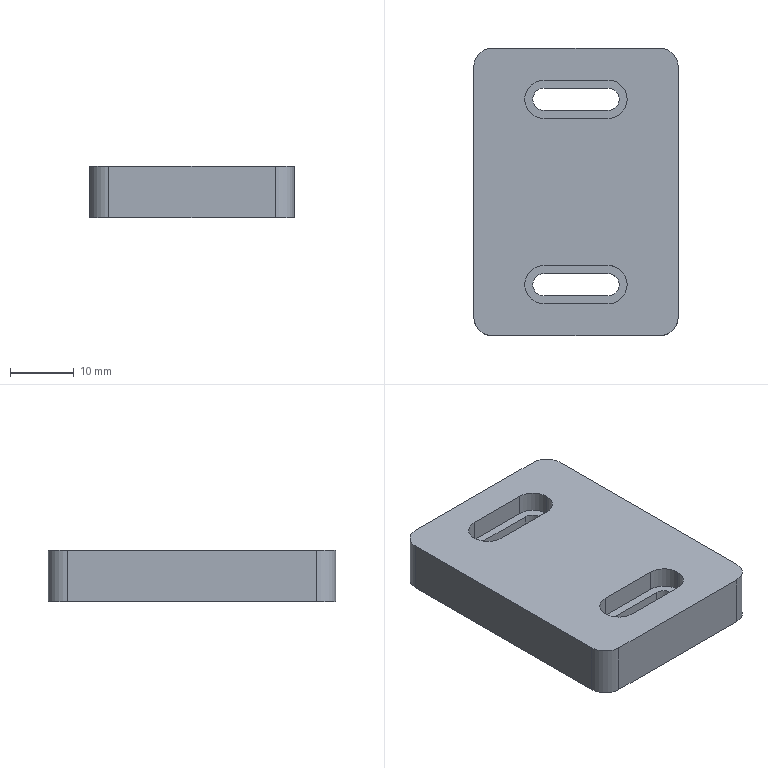Part | SolidWorks | features ICE 2, Extrusion 1, Fillet 1 | 1 solid | 32 faces | box 32 x 45 x 8 mm | volume 10456 mm3 | cylinder 16 | plane 16 | commonest cylinder face diameters 6 x10 3.5 x6
STEP:
#1=CARTESIAN_POINT('',(8.,-14.5,4.7));
#2=VERTEX_POINT('',#1);
#3=CARTESIAN_POINT('',(5.,-11.5,4.7));
#4=VERTEX_POINT('',#3);
#5=CARTESIAN_POINT('',(5.,-14.5,4.7));
#6=DIRECTION('',(0.,0.,1.));
#7=DIRECTION('',(1.,0.,0.));
#8=AXIS2_PLACEMENT_3D('',#5,#6,#7);
#9=CIRCLE('',#8,3.);
#10=EDGE_CURVE('',#2,#4,#9,.T.);
#11=ORIENTED_EDGE('',*,*,#10,.F.);
#12=CARTESIAN_POINT('',(8.,-14.5,8.));
#13=VERTEX_POINT('',#12);
#14=CARTESIAN_POINT('',(8.,-14.5,4.7));
#15=DIRECTION('',(0.,0.,1.));
#16=VECTOR('',#15,1000.);
#17=LINE('',#14,#16);
#18=EDGE_CURVE('',#2,#13,#17,.T.);
#19=ORIENTED_EDGE('',*,*,#18,.T.);
#20=CARTESIAN_POINT('',(5.,-11.5,8.));
#21=VERTEX_POINT('',#20);
#22=CARTESIAN_POINT('',(5.,-14.5,8.));
#23=DIRECTION('',(0.,0.,1.));
#24=DIRECTION('',(1.,0.,0.));
#25=AXIS2_PLACEMENT_3D('',#22,#23,#24);
#26=CIRCLE('',#25,3.);
#27=EDGE_CURVE('',#13,#21,#26,.T.);
#28=ORIENTED_EDGE('',*,*,#27,.T.);
#29=CARTESIAN_POINT('',(5.,-11.5,4.7));
#30=DIRECTION('',(0.,0.,1.));
#31=VECTOR('',#30,1000.);
#32=LINE('',#29,#31);
#33=EDGE_CURVE('',#4,#21,#32,.T.);
#34=ORIENTED_EDGE('',*,*,#33,.F.);
#35=EDGE_LOOP('',(#11,#19,#28,#34));
#36=FACE_OUTER_BOUND('',#35,.T.);
#37=CARTESIAN_POINT('',(5.,-14.5,4.7));
#38=DIRECTION('',(0.,0.,1.));
#39=DIRECTION('',(1.,0.,0.));
#40=AXIS2_PLACEMENT_3D('',#37,#38,#39);
#41=CYLINDRICAL_SURFACE('',#40,3.);
#42=ADVANCED_FACE('',(#36),#41,.F.);
#43=CARTESIAN_POINT('',(8.,14.5,4.7));
#44=VERTEX_POINT('',#43);
#45=CARTESIAN_POINT('',(5.,17.5,4.7));
#46=VERTEX_POINT('',#45);
#47=CARTESIAN_POINT('',(5.,14.5,4.7));
#48=DIRECTION('',(0.,0.,1.));
#49=DIRECTION('',(1.,0.,0.));
#50=AXIS2_PLACEMENT_3D('',#47,#48,#49);
#51=CIRCLE('',#50,3.);
#52=EDGE_CURVE('',#44,#46,#51,.T.);
#53=ORIENTED_EDGE('',*,*,#52,.F.);
#54=CARTESIAN_POINT('',(8.,14.5,8.));
#55=VERTEX_POINT('',#54);
#56=CARTESIAN_POINT('',(8.,14.5,4.7));
#57=DIRECTION('',(0.,0.,1.));
#58=VECTOR('',#57,1000.);
#59=LINE('',#56,#58);
#60=EDGE_CURVE('',#44,#55,#59,.T.);
#61=ORIENTED_EDGE('',*,*,#60,.T.);
#62=CARTESIAN_POINT('',(5.,17.5,8.));
#63=VERTEX_POINT('',#62);
#64=CARTESIAN_POINT('',(5.,14.5,8.));
#65=DIRECTION('',(0.,0.,1.));
#66=DIRECTION('',(1.,0.,0.));
#67=AXIS2_PLACEMENT_3D('',#64,#65,#66);
#68=CIRCLE('',#67,3.);
#69=EDGE_CURVE('',#55,#63,#68,.T.);
#70=ORIENTED_EDGE('',*,*,#69,.T.);
#71=CARTESIAN_POINT('',(5.,17.5,4.7));
#72=DIRECTION('',(0.,0.,1.));
#73=VECTOR('',#72,1000.);
#74=LINE('',#71,#73);
#75=EDGE_CURVE('',#46,#63,#74,.T.);
#76=ORIENTED_EDGE('',*,*,#75,.F.);
#77=EDGE_LOOP('',(#53,#61,#70,#76));
#78=FACE_OUTER_BOUND('',#77,.T.);
#79=CARTESIAN_POINT('',(5.,14.5,4.7));
#80=DIRECTION('',(0.,0.,1.));
#81=DIRECTION('',(1.,0.,0.));
#82=AXIS2_PLACEMENT_3D('',#79,#80,#81);
#83=CYLINDRICAL_SURFACE('',#82,3.);
#84=ADVANCED_FACE('',(#78),#83,.F.);
#85=CARTESIAN_POINT('',(6.75,14.5,0.));
#86=VERTEX_POINT('',#85);
#87=CARTESIAN_POINT('',(5.,16.25,0.));
#88=VERTEX_POINT('',#87);
#89=CARTESIAN_POINT('',(5.,14.5,0.));
#90=DIRECTION('',(0.,0.,1.));
#91=DIRECTION('',(1.,0.,0.));
#92=AXIS2_PLACEMENT_3D('',#89,#90,#91);
#93=CIRCLE('',#92,1.75);
#94=EDGE_CURVE('',#86,#88,#93,.T.);
#95=ORIENTED_EDGE('',*,*,#94,.F.);
#96=CARTESIAN_POINT('',(6.75,14.5,4.7));
#97=VERTEX_POINT('',#96);
#98=CARTESIAN_POINT('',(6.75,14.5,0.));
#99=DIRECTION('',(0.,0.,1.));
#100=VECTOR('',#99,1000.);
#101=LINE('',#98,#100);
#102=EDGE_CURVE('',#86,#97,#101,.T.);
#103=ORIENTED_EDGE('',*,*,#102,.T.);
#104=CARTESIAN_POINT('',(5.,16.25,4.7));
#105=VERTEX_POINT('',#104);
#106=CARTESIAN_POINT('',(5.,14.5,4.7));
#107=DIRECTION('',(0.,0.,-1.));
#108=DIRECTION('',(1.,0.,0.));
#109=AXIS2_PLACEMENT_3D('',#106,#107,#108);
#110=CIRCLE('',#109,1.75);
#111=EDGE_CURVE('',#105,#97,#110,.T.);
#112=ORIENTED_EDGE('',*,*,#111,.F.);
#113=CARTESIAN_POINT('',(5.,16.25,0.));
#114=DIRECTION('',(0.,0.,1.));
#115=VECTOR('',#114,1000.);
#116=LINE('',#113,#115);
#117=EDGE_CURVE('',#88,#105,#116,.T.);
#118=ORIENTED_EDGE('',*,*,#117,.F.);
#119=EDGE_LOOP('',(#95,#103,#112,#118));
#120=FACE_OUTER_BOUND('',#119,.T.);
#121=CARTESIAN_POINT('',(5.,14.5,0.));
#122=DIRECTION('',(0.,0.,1.));
#123=DIRECTION('',(1.,0.,0.));
#124=AXIS2_PLACEMENT_3D('',#121,#122,#123);
#125=CYLINDRICAL_SURFACE('',#124,1.75);
#126=ADVANCED_FACE('',(#120),#125,.F.);
#127=CARTESIAN_POINT('',(6.75,-14.5,0.));
#128=VERTEX_POINT('',#127);
#129=CARTESIAN_POINT('',(5.,-12.75,0.));
#130=VERTEX_POINT('',#129);
#131=CARTESIAN_POINT('',(5.,-14.5,0.));
#132=DIRECTION('',(0.,0.,1.));
#133=DIRECTION('',(1.,0.,0.));
#134=AXIS2_PLACEMENT_3D('',#131,#132,#133);
#135=CIRCLE('',#134,1.75);
#136=EDGE_CURVE('',#128,#130,#135,.T.);
#137=ORIENTED_EDGE('',*,*,#136,.F.);
#138=CARTESIAN_POINT('',(6.75,-14.5,4.7));
#139=VERTEX_POINT('',#138);
#140=CARTESIAN_POINT('',(6.75,-14.5,0.));
#141=DIRECTION('',(0.,0.,1.));
#142=VECTOR('',#141,1000.);
#143=LINE('',#140,#142);
#144=EDGE_CURVE('',#128,#139,#143,.T.);
#145=ORIENTED_EDGE('',*,*,#144,.T.);
#146=CARTESIAN_POINT('',(5.,-12.75,4.7));
#147=VERTEX_POINT('',#146);
#148=CARTESIAN_POINT('',(5.,-14.5,4.7));
#149=DIRECTION('',(0.,0.,-1.));
#150=DIRECTION('',(1.,0.,0.));
#151=AXIS2_PLACEMENT_3D('',#148,#149,#150);
#152=CIRCLE('',#151,1.75);
#153=EDGE_CURVE('',#147,#139,#152,.T.);
#154=ORIENTED_EDGE('',*,*,#153,.F.);
#155=CARTESIAN_POINT('',(5.,-12.75,0.));
#156=DIRECTION('',(0.,0.,1.));
#157=VECTOR('',#156,1000.);
#158=LINE('',#155,#157);
#159=EDGE_CURVE('',#130,#147,#158,.T.);
#160=ORIENTED_EDGE('',*,*,#159,.F.);
#161=EDGE_LOOP('',(#137,#145,#154,#160));
#162=FACE_OUTER_BOUND('',#161,.T.);
#163=CARTESIAN_POINT('',(5.,-14.5,0.));
#164=DIRECTION('',(0.,0.,1.));
#165=DIRECTION('',(1.,0.,0.));
#166=AXIS2_PLACEMENT_3D('',#163,#164,#165);
#167=CYLINDRICAL_SURFACE('',#166,1.75);
#168=ADVANCED_FACE('',(#162),#167,.F.);
#169=CARTESIAN_POINT('',(-5.,-16.25,4.7));
#170=VERTEX_POINT('',#169);
#171=CARTESIAN_POINT('',(-5.,-12.75,4.7));
#172=VERTEX_POINT('',#171);
#173=CARTESIAN_POINT('',(-5.,-14.5,4.7));
#174=DIRECTION('',(0.,0.,-1.));
#175=DIRECTION('',(1.,0.,0.));
#176=AXIS2_PLACEMENT_3D('',#173,#174,#175);
#177=CIRCLE('',#176,1.75);
#178=EDGE_CURVE('',#170,#172,#177,.T.);
#179=ORIENTED_EDGE('',*,*,#178,.F.);
#180=CARTESIAN_POINT('',(-5.,-16.25,0.));
#181=VERTEX_POINT('',#180);
#182=CARTESIAN_POINT('',(-5.,-16.25,0.));
#183=DIRECTION('',(0.,0.,1.));
#184=VECTOR('',#183,1000.);
#185=LINE('',#182,#184);
#186=EDGE_CURVE('',#181,#170,#185,.T.);
#187=ORIENTED_EDGE('',*,*,#186,.F.);
#188=CARTESIAN_POINT('',(-5.,-12.75,0.));
#189=VERTEX_POINT('',#188);
#190=CARTESIAN_POINT('',(-5.,-14.5,0.));
#191=DIRECTION('',(0.,0.,1.));
#192=DIRECTION('',(1.,0.,0.));
#193=AXIS2_PLACEMENT_3D('',#190,#191,#192);
#194=CIRCLE('',#193,1.75);
#195=EDGE_CURVE('',#189,#181,#194,.T.);
#196=ORIENTED_EDGE('',*,*,#195,.F.);
#197=CARTESIAN_POINT('',(-5.,-12.75,0.));
#198=DIRECTION('',(0.,0.,1.));
#199=VECTOR('',#198,1000.);
#200=LINE('',#197,#199);
#201=EDGE_CURVE('',#189,#172,#200,.T.);
#202=ORIENTED_EDGE('',*,*,#201,.T.);
#203=EDGE_LOOP('',(#179,#187,#196,#202));
#204=FACE_OUTER_BOUND('',#203,.T.);
#205=CARTESIAN_POINT('',(-5.,-14.5,0.));
#206=DIRECTION('',(0.,0.,1.));
#207=DIRECTION('',(1.,0.,0.));
#208=AXIS2_PLACEMENT_3D('',#205,#206,#207);
#209=CYLINDRICAL_SURFACE('',#208,1.75);
#210=ADVANCED_FACE('',(#204),#209,.F.);
#211=CARTESIAN_POINT('',(-5.,-12.75,4.7));
#212=DIRECTION('',(1.,0.,0.));
#213=VECTOR('',#212,1000.);
#214=LINE('',#211,#213);
#215=EDGE_CURVE('',#172,#147,#214,.T.);
#216=ORIENTED_EDGE('',*,*,#215,.F.);
#217=ORIENTED_EDGE('',*,*,#201,.F.);
#218=CARTESIAN_POINT('',(-5.,-12.75,0.));
#219=DIRECTION('',(-1.,0.,0.));
#220=VECTOR('',#219,1000.);
#221=LINE('',#218,#220);
#222=EDGE_CURVE('',#130,#189,#221,.T.);
#223=ORIENTED_EDGE('',*,*,#222,.F.);
#224=ORIENTED_EDGE('',*,*,#159,.T.);
#225=EDGE_LOOP('',(#216,#217,#223,#224));
#226=FACE_OUTER_BOUND('',#225,.T.);
#227=CARTESIAN_POINT('',(-5.,-12.75,0.));
#228=DIRECTION('',(0.,1.,0.));
#229=DIRECTION('',(-1.,0.,0.));
#230=AXIS2_PLACEMENT_3D('',#227,#228,#229);
#231=PLANE('',#230);
#232=ADVANCED_FACE('',(#226),#231,.F.);
#233=ORIENTED_EDGE('',*,*,#144,.F.);
#234=CARTESIAN_POINT('',(5.,-16.25,0.));
#235=VERTEX_POINT('',#234);
#236=CARTESIAN_POINT('',(5.,-14.5,0.));
#237=DIRECTION('',(0.,0.,1.));
#238=DIRECTION('',(1.,0.,0.));
#239=AXIS2_PLACEMENT_3D('',#236,#237,#238);
#240=CIRCLE('',#239,1.75);
#241=EDGE_CURVE('',#235,#128,#240,.T.);
#242=ORIENTED_EDGE('',*,*,#241,.F.);
#243=CARTESIAN_POINT('',(5.,-16.25,4.7));
#244=VERTEX_POINT('',#243);
#245=CARTESIAN_POINT('',(5.,-16.25,0.));
#246=DIRECTION('',(0.,0.,1.));
#247=VECTOR('',#246,1000.);
#248=LINE('',#245,#247);
#249=EDGE_CURVE('',#235,#244,#248,.T.);
#250=ORIENTED_EDGE('',*,*,#249,.T.);
#251=CARTESIAN_POINT('',(5.,-14.5,4.7));
#252=DIRECTION('',(0.,0.,-1.));
#253=DIRECTION('',(1.,0.,0.));
#254=AXIS2_PLACEMENT_3D('',#251,#252,#253);
#255=CIRCLE('',#254,1.75);
#256=EDGE_CURVE('',#139,#244,#255,.T.);
#257=ORIENTED_EDGE('',*,*,#256,.F.);
#258=EDGE_LOOP('',(#233,#242,#250,#257));
#259=FACE_OUTER_BOUND('',#258,.T.);
#260=CARTESIAN_POINT('',(5.,-14.5,0.));
#261=DIRECTION('',(0.,0.,1.));
#262=DIRECTION('',(1.,0.,0.));
#263=AXIS2_PLACEMENT_3D('',#260,#261,#262);
#264=CYLINDRICAL_SURFACE('',#263,1.75);
#265=ADVANCED_FACE('',(#259),#264,.F.);
#266=CARTESIAN_POINT('',(-5.,-16.25,4.7));
#267=DIRECTION('',(-1.,0.,0.));
#268=VECTOR('',#267,1000.);
#269=LINE('',#266,#268);
#270=EDGE_CURVE('',#244,#170,#269,.T.);
#271=ORIENTED_EDGE('',*,*,#270,.F.);
#272=ORIENTED_EDGE('',*,*,#249,.F.);
#273=CARTESIAN_POINT('',(-5.,-16.25,0.));
#274=DIRECTION('',(1.,0.,0.));
#275=VECTOR('',#274,1000.);
#276=LINE('',#273,#275);
#277=EDGE_CURVE('',#181,#235,#276,.T.);
#278=ORIENTED_EDGE('',*,*,#277,.F.);
#279=ORIENTED_EDGE('',*,*,#186,.T.);
#280=EDGE_LOOP('',(#271,#272,#278,#279));
#281=FACE_OUTER_BOUND('',#280,.T.);
#282=CARTESIAN_POINT('',(-5.,-16.25,0.));
#283=DIRECTION('',(0.,-1.,0.));
#284=DIRECTION('',(0.,0.,-1.));
#285=AXIS2_PLACEMENT_3D('',#282,#283,#284);
#286=PLANE('',#285);
#287=ADVANCED_FACE('',(#281),#286,.F.);
#288=CARTESIAN_POINT('',(-5.,12.75,4.7));
#289=VERTEX_POINT('',#288);
#290=CARTESIAN_POINT('',(-5.,16.25,4.7));
#291=VERTEX_POINT('',#290);
#292=CARTESIAN_POINT('',(-5.,14.5,4.7));
#293=DIRECTION('',(0.,0.,-1.));
#294=DIRECTION('',(1.,0.,0.));
#295=AXIS2_PLACEMENT_3D('',#292,#293,#294);
#296=CIRCLE('',#295,1.75);
#297=EDGE_CURVE('',#289,#291,#296,.T.);
#298=ORIENTED_EDGE('',*,*,#297,.F.);
#299=CARTESIAN_POINT('',(-5.,12.75,0.));
#300=VERTEX_POINT('',#299);
#301=CARTESIAN_POINT('',(-5.,12.75,0.));
#302=DIRECTION('',(0.,0.,1.));
#303=VECTOR('',#302,1000.);
#304=LINE('',#301,#303);
#305=EDGE_CURVE('',#300,#289,#304,.T.);
#306=ORIENTED_EDGE('',*,*,#305,.F.);
#307=CARTESIAN_POINT('',(-5.,16.25,0.));
#308=VERTEX_POINT('',#307);
#309=CARTESIAN_POINT('',(-5.,14.5,0.));
#310=DIRECTION('',(0.,0.,1.));
#311=DIRECTION('',(1.,0.,0.));
#312=AXIS2_PLACEMENT_3D('',#309,#310,#311);
#313=CIRCLE('',#312,1.75);
#314=EDGE_CURVE('',#308,#300,#313,.T.);
#315=ORIENTED_EDGE('',*,*,#314,.F.);
#316=CARTESIAN_POINT('',(-5.,16.25,0.));
#317=DIRECTION('',(0.,0.,1.));
#318=VECTOR('',#317,1000.);
#319=LINE('',#316,#318);
#320=EDGE_CURVE('',#308,#291,#319,.T.);
#321=ORIENTED_EDGE('',*,*,#320,.T.);
#322=EDGE_LOOP('',(#298,#306,#315,#321));
#323=FACE_OUTER_BOUND('',#322,.T.);
#324=CARTESIAN_POINT('',(-5.,14.5,0.));
#325=DIRECTION('',(0.,0.,1.));
#326=DIRECTION('',(1.,0.,0.));
#327=AXIS2_PLACEMENT_3D('',#324,#325,#326);
#328=CYLINDRICAL_SURFACE('',#327,1.75);
#329=ADVANCED_FACE('',(#323),#328,.F.);
#330=CARTESIAN_POINT('',(-5.,16.25,4.7));
#331=DIRECTION('',(1.,0.,0.));
#332=VECTOR('',#331,1000.);
#333=LINE('',#330,#332);
#334=EDGE_CURVE('',#291,#105,#333,.T.);
#335=ORIENTED_EDGE('',*,*,#334,.F.);
#336=ORIENTED_EDGE('',*,*,#320,.F.);
#337=CARTESIAN_POINT('',(-5.,16.25,0.));
#338=DIRECTION('',(-1.,0.,0.));
#339=VECTOR('',#338,1000.);
#340=LINE('',#337,#339);
#341=EDGE_CURVE('',#88,#308,#340,.T.);
#342=ORIENTED_EDGE('',*,*,#341,.F.);
#343=ORIENTED_EDGE('',*,*,#117,.T.);
#344=EDGE_LOOP('',(#335,#336,#342,#343));
#345=FACE_OUTER_BOUND('',#344,.T.);
#346=CARTESIAN_POINT('',(-5.,16.25,0.));
#347=DIRECTION('',(0.,1.,0.));
#348=DIRECTION('',(-1.,0.,0.));
#349=AXIS2_PLACEMENT_3D('',#346,#347,#348);
#350=PLANE('',#349);
#351=ADVANCED_FACE('',(#345),#350,.F.);
#352=ORIENTED_EDGE('',*,*,#102,.F.);
#353=CARTESIAN_POINT('',(5.,12.75,0.));
#354=VERTEX_POINT('',#353);
#355=CARTESIAN_POINT('',(5.,14.5,0.));
#356=DIRECTION('',(0.,0.,1.));
#357=DIRECTION('',(1.,0.,0.));
#358=AXIS2_PLACEMENT_3D('',#355,#356,#357);
#359=CIRCLE('',#358,1.75);
#360=EDGE_CURVE('',#354,#86,#359,.T.);
#361=ORIENTED_EDGE('',*,*,#360,.F.);
#362=CARTESIAN_POINT('',(5.,12.75,4.7));
#363=VERTEX_POINT('',#362);
#364=CARTESIAN_POINT('',(5.,12.75,0.));
#365=DIRECTION('',(0.,0.,1.));
#366=VECTOR('',#365,1000.);
#367=LINE('',#364,#366);
#368=EDGE_CURVE('',#354,#363,#367,.T.);
#369=ORIENTED_EDGE('',*,*,#368,.T.);
#370=CARTESIAN_POINT('',(5.,14.5,4.7));
#371=DIRECTION('',(0.,0.,-1.));
#372=DIRECTION('',(1.,0.,0.));
#373=AXIS2_PLACEMENT_3D('',#370,#371,#372);
#374=CIRCLE('',#373,1.75);
#375=EDGE_CURVE('',#97,#363,#374,.T.);
#376=ORIENTED_EDGE('',*,*,#375,.F.);
#377=EDGE_LOOP('',(#352,#361,#369,#376));
#378=FACE_OUTER_BOUND('',#377,.T.);
#379=CARTESIAN_POINT('',(5.,14.5,0.));
#380=DIRECTION('',(0.,0.,1.));
#381=DIRECTION('',(1.,0.,0.));
#382=AXIS2_PLACEMENT_3D('',#379,#380,#381);
#383=CYLINDRICAL_SURFACE('',#382,1.75);
#384=ADVANCED_FACE('',(#378),#383,.F.);
#385=CARTESIAN_POINT('',(-5.,12.75,4.7));
#386=DIRECTION('',(-1.,0.,0.));
#387=VECTOR('',#386,1000.);
#388=LINE('',#385,#387);
#389=EDGE_CURVE('',#363,#289,#388,.T.);
#390=ORIENTED_EDGE('',*,*,#389,.F.);
#391=ORIENTED_EDGE('',*,*,#368,.F.);
#392=CARTESIAN_POINT('',(-5.,12.75,0.));
#393=DIRECTION('',(1.,0.,0.));
#394=VECTOR('',#393,1000.);
#395=LINE('',#392,#394);
#396=EDGE_CURVE('',#300,#354,#395,.T.);
#397=ORIENTED_EDGE('',*,*,#396,.F.);
#398=ORIENTED_EDGE('',*,*,#305,.T.);
#399=EDGE_LOOP('',(#390,#391,#397,#398));
#400=FACE_OUTER_BOUND('',#399,.T.);
#401=CARTESIAN_POINT('',(-5.,12.75,0.));
#402=DIRECTION('',(0.,-1.,0.));
#403=DIRECTION('',(0.,0.,-1.));
#404=AXIS2_PLACEMENT_3D('',#401,#402,#403);
#405=PLANE('',#404);
#406=ADVANCED_FACE('',(#400),#405,.F.);
#407=CARTESIAN_POINT('',(-16.,19.5,0.));
#408=VERTEX_POINT('',#407);
#409=CARTESIAN_POINT('',(-16.,-19.5,0.));
#410=VERTEX_POINT('',#409);
#411=CARTESIAN_POINT('',(-16.,-22.5,0.));
#412=DIRECTION('',(0.,-1.,0.));
#413=VECTOR('',#412,1000.);
#414=LINE('',#411,#413);
#415=EDGE_CURVE('',#408,#410,#414,.T.);
#416=ORIENTED_EDGE('',*,*,#415,.T.);
#417=CARTESIAN_POINT('',(-16.,-19.5,8.));
#418=VERTEX_POINT('',#417);
#419=CARTESIAN_POINT('',(-16.,-19.5,8.));
#420=DIRECTION('',(0.,0.,1.));
#421=VECTOR('',#420,1000.);
#422=LINE('',#419,#421);
#423=EDGE_CURVE('',#410,#418,#422,.T.);
#424=ORIENTED_EDGE('',*,*,#423,.T.);
#425=CARTESIAN_POINT('',(-16.,19.5,8.));
#426=VERTEX_POINT('',#425);
#427=CARTESIAN_POINT('',(-16.,-22.5,8.));
#428=DIRECTION('',(0.,-1.,0.));
#429=VECTOR('',#428,1000.);
#430=LINE('',#427,#429);
#431=EDGE_CURVE('',#426,#418,#430,.T.);
#432=ORIENTED_EDGE('',*,*,#431,.F.);
#433=CARTESIAN_POINT('',(-16.,19.5,8.));
#434=DIRECTION('',(0.,0.,-1.));
#435=VECTOR('',#434,1000.);
#436=LINE('',#433,#435);
#437=EDGE_CURVE('',#426,#408,#436,.T.);
#438=ORIENTED_EDGE('',*,*,#437,.T.);
#439=EDGE_LOOP('',(#416,#424,#432,#438));
#440=FACE_OUTER_BOUND('',#439,.T.);
#441=CARTESIAN_POINT('',(-16.,-22.5,8.));
#442=DIRECTION('',(1.,0.,0.));
#443=DIRECTION('',(0.,0.,-1.));
#444=AXIS2_PLACEMENT_3D('',#441,#442,#443);
#445=PLANE('',#444);
#446=ADVANCED_FACE('',(#440),#445,.F.);
#447=CARTESIAN_POINT('',(-13.,-22.5,8.));
#448=VERTEX_POINT('',#447);
#449=CARTESIAN_POINT('',(13.,-22.5,8.));
#450=VERTEX_POINT('',#449);
#451=CARTESIAN_POINT('',(16.,-22.5,8.));
#452=DIRECTION('',(1.,0.,0.));
#453=VECTOR('',#452,1000.);
#454=LINE('',#451,#453);
#455=EDGE_CURVE('',#448,#450,#454,.T.);
#456=ORIENTED_EDGE('',*,*,#455,.F.);
#457=CARTESIAN_POINT('',(-13.,-22.5,0.));
#458=VERTEX_POINT('',#457);
#459=CARTESIAN_POINT('',(-13.,-22.5,8.));
#460=DIRECTION('',(0.,0.,-1.));
#461=VECTOR('',#460,1000.);
#462=LINE('',#459,#461);
#463=EDGE_CURVE('',#448,#458,#462,.T.);
#464=ORIENTED_EDGE('',*,*,#463,.T.);
#465=CARTESIAN_POINT('',(13.,-22.5,0.));
#466=VERTEX_POINT('',#465);
#467=CARTESIAN_POINT('',(16.,-22.5,0.));
#468=DIRECTION('',(1.,0.,0.));
#469=VECTOR('',#468,1000.);
#470=LINE('',#467,#469);
#471=EDGE_CURVE('',#458,#466,#470,.T.);
#472=ORIENTED_EDGE('',*,*,#471,.T.);
#473=CARTESIAN_POINT('',(13.,-22.5,8.));
#474=DIRECTION('',(0.,0.,1.));
#475=VECTOR('',#474,1000.);
#476=LINE('',#473,#475);
#477=EDGE_CURVE('',#466,#450,#476,.T.);
#478=ORIENTED_EDGE('',*,*,#477,.T.);
#479=EDGE_LOOP('',(#456,#464,#472,#478));
#480=FACE_OUTER_BOUND('',#479,.T.);
#481=CARTESIAN_POINT('',(16.,-22.5,8.));
#482=DIRECTION('',(0.,1.,0.));
#483=DIRECTION('',(-1.,0.,0.));
#484=AXIS2_PLACEMENT_3D('',#481,#482,#483);
#485=PLANE('',#484);
#486=ADVANCED_FACE('',(#480),#485,.F.);
#487=CARTESIAN_POINT('',(16.,-19.5,8.));
#488=VERTEX_POINT('',#487);
#489=CARTESIAN_POINT('',(16.,19.5,8.));
#490=VERTEX_POINT('',#489);
#491=CARTESIAN_POINT('',(16.,-22.5,8.));
#492=DIRECTION('',(0.,1.,0.));
#493=VECTOR('',#492,1000.);
#494=LINE('',#491,#493);
#495=EDGE_CURVE('',#488,#490,#494,.T.);
#496=ORIENTED_EDGE('',*,*,#495,.F.);
#497=CARTESIAN_POINT('',(16.,-19.5,0.));
#498=VERTEX_POINT('',#497);
#499=CARTESIAN_POINT('',(16.,-19.5,8.));
#500=DIRECTION('',(0.,0.,-1.));
#501=VECTOR('',#500,1000.);
#502=LINE('',#499,#501);
#503=EDGE_CURVE('',#488,#498,#502,.T.);
#504=ORIENTED_EDGE('',*,*,#503,.T.);
#505=CARTESIAN_POINT('',(16.,19.5,0.));
#506=VERTEX_POINT('',#505);
#507=CARTESIAN_POINT('',(16.,-22.5,0.));
#508=DIRECTION('',(0.,1.,0.));
#509=VECTOR('',#508,1000.);
#510=LINE('',#507,#509);
#511=EDGE_CURVE('',#498,#506,#510,.T.);
#512=ORIENTED_EDGE('',*,*,#511,.T.);
#513=CARTESIAN_POINT('',(16.,19.5,8.));
#514=DIRECTION('',(0.,0.,1.));
#515=VECTOR('',#514,1000.);
#516=LINE('',#513,#515);
#517=EDGE_CURVE('',#506,#490,#516,.T.);
#518=ORIENTED_EDGE('',*,*,#517,.T.);
#519=EDGE_LOOP('',(#496,#504,#512,#518));
#520=FACE_OUTER_BOUND('',#519,.T.);
#521=CARTESIAN_POINT('',(16.,-22.5,8.));
#522=DIRECTION('',(-1.,0.,0.));
#523=DIRECTION('',(0.,0.,1.));
#524=AXIS2_PLACEMENT_3D('',#521,#522,#523);
#525=PLANE('',#524);
#526=ADVANCED_FACE('',(#520),#525,.F.);
#527=CARTESIAN_POINT('',(13.,22.5,8.));
#528=VERTEX_POINT('',#527);
#529=CARTESIAN_POINT('',(-13.,22.5,8.));
#530=VERTEX_POINT('',#529);
#531=CARTESIAN_POINT('',(16.,22.5,8.));
#532=DIRECTION('',(-1.,0.,0.));
#533=VECTOR('',#532,1000.);
#534=LINE('',#531,#533);
#535=EDGE_CURVE('',#528,#530,#534,.T.);
#536=ORIENTED_EDGE('',*,*,#535,.F.);
#537=CARTESIAN_POINT('',(13.,22.5,0.));
#538=VERTEX_POINT('',#537);
#539=CARTESIAN_POINT('',(13.,22.5,8.));
#540=DIRECTION('',(0.,0.,-1.));
#541=VECTOR('',#540,1000.);
#542=LINE('',#539,#541);
#543=EDGE_CURVE('',#528,#538,#542,.T.);
#544=ORIENTED_EDGE('',*,*,#543,.T.);
#545=CARTESIAN_POINT('',(-13.,22.5,0.));
#546=VERTEX_POINT('',#545);
#547=CARTESIAN_POINT('',(16.,22.5,0.));
#548=DIRECTION('',(-1.,0.,0.));
#549=VECTOR('',#548,1000.);
#550=LINE('',#547,#549);
#551=EDGE_CURVE('',#538,#546,#550,.T.);
#552=ORIENTED_EDGE('',*,*,#551,.T.);
#553=CARTESIAN_POINT('',(-13.,22.5,8.));
#554=DIRECTION('',(0.,0.,1.));
#555=VECTOR('',#554,1000.);
#556=LINE('',#553,#555);
#557=EDGE_CURVE('',#546,#530,#556,.T.);
#558=ORIENTED_EDGE('',*,*,#557,.T.);
#559=EDGE_LOOP('',(#536,#544,#552,#558));
#560=FACE_OUTER_BOUND('',#559,.T.);
#561=CARTESIAN_POINT('',(16.,22.5,8.));
#562=DIRECTION('',(0.,-1.,0.));
#563=DIRECTION('',(1.,0.,0.));
#564=AXIS2_PLACEMENT_3D('',#561,#562,#563);
#565=PLANE('',#564);
#566=ADVANCED_FACE('',(#560),#565,.F.);
#567=CARTESIAN_POINT('',(-5.,17.5,8.));
#568=VERTEX_POINT('',#567);
#569=CARTESIAN_POINT('',(-5.,11.5,8.));
#570=VERTEX_POINT('',#569);
#571=CARTESIAN_POINT('',(-5.,14.5,8.));
#572=DIRECTION('',(0.,0.,1.));
#573=DIRECTION('',(1.,0.,0.));
#574=AXIS2_PLACEMENT_3D('',#571,#572,#573);
#575=CIRCLE('',#574,3.);
#576=EDGE_CURVE('',#568,#570,#575,.T.);
#577=ORIENTED_EDGE('',*,*,#576,.F.);
#578=CARTESIAN_POINT('',(-5.,17.5,8.));
#579=DIRECTION('',(-1.,0.,0.));
#580=VECTOR('',#579,1000.);
#581=LINE('',#578,#580);
#582=EDGE_CURVE('',#63,#568,#581,.T.);
#583=ORIENTED_EDGE('',*,*,#582,.F.);
#584=ORIENTED_EDGE('',*,*,#69,.F.);
#585=CARTESIAN_POINT('',(5.,11.5,8.));
#586=VERTEX_POINT('',#585);
#587=CARTESIAN_POINT('',(5.,14.5,8.));
#588=DIRECTION('',(0.,0.,1.));
#589=DIRECTION('',(1.,0.,0.));
#590=AXIS2_PLACEMENT_3D('',#587,#588,#589);
#591=CIRCLE('',#590,3.);
#592=EDGE_CURVE('',#586,#55,#591,.T.);
#593=ORIENTED_EDGE('',*,*,#592,.F.);
#594=CARTESIAN_POINT('',(-5.,11.5,8.));
#595=DIRECTION('',(1.,0.,0.));
#596=VECTOR('',#595,1000.);
#597=LINE('',#594,#596);
#598=EDGE_CURVE('',#570,#586,#597,.T.);
#599=ORIENTED_EDGE('',*,*,#598,.F.);
#600=EDGE_LOOP('',(#577,#583,#584,#593,#599));
#601=FACE_BOUND('',#600,.T.);
#602=CARTESIAN_POINT('',(-5.,-11.5,8.));
#603=VERTEX_POINT('',#602);
#604=CARTESIAN_POINT('',(-5.,-17.5,8.));
#605=VERTEX_POINT('',#604);
#606=CARTESIAN_POINT('',(-5.,-14.5,8.));
#607=DIRECTION('',(0.,0.,1.));
#608=DIRECTION('',(1.,0.,0.));
#609=AXIS2_PLACEMENT_3D('',#606,#607,#608);
#610=CIRCLE('',#609,3.);
#611=EDGE_CURVE('',#603,#605,#610,.T.);
#612=ORIENTED_EDGE('',*,*,#611,.F.);
#613=CARTESIAN_POINT('',(-5.,-11.5,8.));
#614=DIRECTION('',(-1.,0.,0.));
#615=VECTOR('',#614,1000.);
#616=LINE('',#613,#615);
#617=EDGE_CURVE('',#21,#603,#616,.T.);
#618=ORIENTED_EDGE('',*,*,#617,.F.);
#619=ORIENTED_EDGE('',*,*,#27,.F.);
#620=CARTESIAN_POINT('',(5.,-17.5,8.));
#621=VERTEX_POINT('',#620);
#622=CARTESIAN_POINT('',(5.,-14.5,8.));
#623=DIRECTION('',(0.,0.,1.));
#624=DIRECTION('',(1.,0.,0.));
#625=AXIS2_PLACEMENT_3D('',#622,#623,#624);
#626=CIRCLE('',#625,3.);
#627=EDGE_CURVE('',#621,#13,#626,.T.);
#628=ORIENTED_EDGE('',*,*,#627,.F.);
#629=CARTESIAN_POINT('',(-5.,-17.5,8.));
#630=DIRECTION('',(1.,0.,0.));
#631=VECTOR('',#630,1000.);
#632=LINE('',#629,#631);
#633=EDGE_CURVE('',#605,#621,#632,.T.);
#634=ORIENTED_EDGE('',*,*,#633,.F.);
#635=EDGE_LOOP('',(#612,#618,#619,#628,#634));
#636=FACE_BOUND('',#635,.T.);
#637=ORIENTED_EDGE('',*,*,#431,.T.);
#638=CARTESIAN_POINT('',(-13.,-19.5,8.));
#639=DIRECTION('',(0.,0.,1.));
#640=DIRECTION('',(1.,0.,0.));
#641=AXIS2_PLACEMENT_3D('',#638,#639,#640);
#642=CIRCLE('',#641,3.);
#643=EDGE_CURVE('',#418,#448,#642,.T.);
#644=ORIENTED_EDGE('',*,*,#643,.T.);
#645=ORIENTED_EDGE('',*,*,#455,.T.);
#646=CARTESIAN_POINT('',(13.,-19.5,8.));
#647=DIRECTION('',(0.,0.,1.));
#648=DIRECTION('',(1.,0.,0.));
#649=AXIS2_PLACEMENT_3D('',#646,#647,#648);
#650=CIRCLE('',#649,3.);
#651=EDGE_CURVE('',#450,#488,#650,.T.);
#652=ORIENTED_EDGE('',*,*,#651,.T.);
#653=ORIENTED_EDGE('',*,*,#495,.T.);
#654=CARTESIAN_POINT('',(13.,19.5,8.));
#655=DIRECTION('',(0.,0.,1.));
#656=DIRECTION('',(1.,0.,0.));
#657=AXIS2_PLACEMENT_3D('',#654,#655,#656);
#658=CIRCLE('',#657,3.);
#659=EDGE_CURVE('',#490,#528,#658,.T.);
#660=ORIENTED_EDGE('',*,*,#659,.T.);
#661=ORIENTED_EDGE('',*,*,#535,.T.);
#662=CARTESIAN_POINT('',(-13.,19.5,8.));
#663=DIRECTION('',(0.,0.,1.));
#664=DIRECTION('',(1.,0.,0.));
#665=AXIS2_PLACEMENT_3D('',#662,#663,#664);
#666=CIRCLE('',#665,3.);
#667=EDGE_CURVE('',#530,#426,#666,.T.);
#668=ORIENTED_EDGE('',*,*,#667,.T.);
#669=EDGE_LOOP('',(#637,#644,#645,#652,#653,#660,#661,#668));
#670=FACE_OUTER_BOUND('',#669,.T.);
#671=CARTESIAN_POINT('',(0.,0.,8.));
#672=DIRECTION('',(0.,0.,1.));
#673=DIRECTION('',(1.,0.,0.));
#674=AXIS2_PLACEMENT_3D('',#671,#672,#673);
#675=PLANE('',#674);
#676=ADVANCED_FACE('',(#601,#636,#670),#675,.T.);
#677=ORIENTED_EDGE('',*,*,#341,.T.);
#678=ORIENTED_EDGE('',*,*,#314,.T.);
#679=ORIENTED_EDGE('',*,*,#396,.T.);
#680=ORIENTED_EDGE('',*,*,#360,.T.);
#681=ORIENTED_EDGE('',*,*,#94,.T.);
#682=EDGE_LOOP('',(#677,#678,#679,#680,#681));
#683=FACE_BOUND('',#682,.T.);
#684=ORIENTED_EDGE('',*,*,#222,.T.);
#685=ORIENTED_EDGE('',*,*,#195,.T.);
#686=ORIENTED_EDGE('',*,*,#277,.T.);
#687=ORIENTED_EDGE('',*,*,#241,.T.);
#688=ORIENTED_EDGE('',*,*,#136,.T.);
#689=EDGE_LOOP('',(#684,#685,#686,#687,#688));
#690=FACE_BOUND('',#689,.T.);
#691=ORIENTED_EDGE('',*,*,#471,.F.);
#692=CARTESIAN_POINT('',(-13.,-19.5,0.));
#693=DIRECTION('',(0.,0.,-1.));
#694=DIRECTION('',(1.,0.,0.));
#695=AXIS2_PLACEMENT_3D('',#692,#693,#694);
#696=CIRCLE('',#695,3.);
#697=EDGE_CURVE('',#458,#410,#696,.T.);
#698=ORIENTED_EDGE('',*,*,#697,.T.);
#699=ORIENTED_EDGE('',*,*,#415,.F.);
#700=CARTESIAN_POINT('',(-13.,19.5,0.));
#701=DIRECTION('',(0.,0.,-1.));
#702=DIRECTION('',(1.,0.,0.));
#703=AXIS2_PLACEMENT_3D('',#700,#701,#702);
#704=CIRCLE('',#703,3.);
#705=EDGE_CURVE('',#408,#546,#704,.T.);
#706=ORIENTED_EDGE('',*,*,#705,.T.);
#707=ORIENTED_EDGE('',*,*,#551,.F.);
#708=CARTESIAN_POINT('',(13.,19.5,0.));
#709=DIRECTION('',(0.,0.,-1.));
#710=DIRECTION('',(1.,0.,0.));
#711=AXIS2_PLACEMENT_3D('',#708,#709,#710);
#712=CIRCLE('',#711,3.);
#713=EDGE_CURVE('',#538,#506,#712,.T.);
#714=ORIENTED_EDGE('',*,*,#713,.T.);
#715=ORIENTED_EDGE('',*,*,#511,.F.);
#716=CARTESIAN_POINT('',(13.,-19.5,0.));
#717=DIRECTION('',(0.,0.,-1.));
#718=DIRECTION('',(1.,0.,0.));
#719=AXIS2_PLACEMENT_3D('',#716,#717,#718);
#720=CIRCLE('',#719,3.);
#721=EDGE_CURVE('',#498,#466,#720,.T.);
#722=ORIENTED_EDGE('',*,*,#721,.T.);
#723=EDGE_LOOP('',(#691,#698,#699,#706,#707,#714,#715,#722));
#724=FACE_OUTER_BOUND('',#723,.T.);
#725=CARTESIAN_POINT('',(0.,0.,0.));
#726=DIRECTION('',(0.,0.,1.));
#727=DIRECTION('',(1.,0.,0.));
#728=AXIS2_PLACEMENT_3D('',#725,#726,#727);
#729=PLANE('',#728);
#730=ADVANCED_FACE('',(#683,#690,#724),#729,.F.);
#731=ORIENTED_EDGE('',*,*,#643,.F.);
#732=ORIENTED_EDGE('',*,*,#423,.F.);
#733=ORIENTED_EDGE('',*,*,#697,.F.);
#734=ORIENTED_EDGE('',*,*,#463,.F.);
#735=EDGE_LOOP('',(#731,#732,#733,#734));
#736=FACE_OUTER_BOUND('',#735,.T.);
#737=CARTESIAN_POINT('',(-13.,-19.5,8.));
#738=DIRECTION('',(0.,0.,-1.));
#739=DIRECTION('',(-1.,0.,0.));
#740=AXIS2_PLACEMENT_3D('',#737,#738,#739);
#741=CYLINDRICAL_SURFACE('',#740,3.);
#742=ADVANCED_FACE('',(#736),#741,.T.);
#743=ORIENTED_EDGE('',*,*,#651,.F.);
#744=ORIENTED_EDGE('',*,*,#477,.F.);
#745=ORIENTED_EDGE('',*,*,#721,.F.);
#746=ORIENTED_EDGE('',*,*,#503,.F.);
#747=EDGE_LOOP('',(#743,#744,#745,#746));
#748=FACE_OUTER_BOUND('',#747,.T.);
#749=CARTESIAN_POINT('',(13.,-19.5,8.));
#750=DIRECTION('',(0.,0.,-1.));
#751=DIRECTION('',(-1.,0.,0.));
#752=AXIS2_PLACEMENT_3D('',#749,#750,#751);
#753=CYLINDRICAL_SURFACE('',#752,3.);
#754=ADVANCED_FACE('',(#748),#753,.T.);
#755=ORIENTED_EDGE('',*,*,#659,.F.);
#756=ORIENTED_EDGE('',*,*,#517,.F.);
#757=ORIENTED_EDGE('',*,*,#713,.F.);
#758=ORIENTED_EDGE('',*,*,#543,.F.);
#759=EDGE_LOOP('',(#755,#756,#757,#758));
#760=FACE_OUTER_BOUND('',#759,.T.);
#761=CARTESIAN_POINT('',(13.,19.5,8.));
#762=DIRECTION('',(0.,0.,-1.));
#763=DIRECTION('',(-1.,0.,0.));
#764=AXIS2_PLACEMENT_3D('',#761,#762,#763);
#765=CYLINDRICAL_SURFACE('',#764,3.);
#766=ADVANCED_FACE('',(#760),#765,.T.);
#767=ORIENTED_EDGE('',*,*,#667,.F.);
#768=ORIENTED_EDGE('',*,*,#557,.F.);
#769=ORIENTED_EDGE('',*,*,#705,.F.);
#770=ORIENTED_EDGE('',*,*,#437,.F.);
#771=EDGE_LOOP('',(#767,#768,#769,#770));
#772=FACE_OUTER_BOUND('',#771,.T.);
#773=CARTESIAN_POINT('',(-13.,19.5,8.));
#774=DIRECTION('',(0.,0.,-1.));
#775=DIRECTION('',(-1.,0.,0.));
#776=AXIS2_PLACEMENT_3D('',#773,#774,#775);
#777=CYLINDRICAL_SURFACE('',#776,3.);
#778=ADVANCED_FACE('',(#772),#777,.T.);
#779=CARTESIAN_POINT('',(-5.,17.5,4.7));
#780=VERTEX_POINT('',#779);
#781=CARTESIAN_POINT('',(-5.,11.5,4.7));
#782=VERTEX_POINT('',#781);
#783=CARTESIAN_POINT('',(-5.,14.5,4.7));
#784=DIRECTION('',(0.,0.,1.));
#785=DIRECTION('',(1.,0.,0.));
#786=AXIS2_PLACEMENT_3D('',#783,#784,#785);
#787=CIRCLE('',#786,3.);
#788=EDGE_CURVE('',#780,#782,#787,.T.);
#789=ORIENTED_EDGE('',*,*,#788,.T.);
#790=CARTESIAN_POINT('',(5.,11.5,4.7));
#791=VERTEX_POINT('',#790);
#792=CARTESIAN_POINT('',(-5.,11.5,4.7));
#793=DIRECTION('',(1.,0.,0.));
#794=VECTOR('',#793,1000.);
#795=LINE('',#792,#794);
#796=EDGE_CURVE('',#782,#791,#795,.T.);
#797=ORIENTED_EDGE('',*,*,#796,.T.);
#798=CARTESIAN_POINT('',(5.,14.5,4.7));
#799=DIRECTION('',(0.,0.,1.));
#800=DIRECTION('',(1.,0.,0.));
#801=AXIS2_PLACEMENT_3D('',#798,#799,#800);
#802=CIRCLE('',#801,3.);
#803=EDGE_CURVE('',#791,#44,#802,.T.);
#804=ORIENTED_EDGE('',*,*,#803,.T.);
#805=ORIENTED_EDGE('',*,*,#52,.T.);
#806=CARTESIAN_POINT('',(-5.,17.5,4.7));
#807=DIRECTION('',(-1.,0.,0.));
#808=VECTOR('',#807,1000.);
#809=LINE('',#806,#808);
#810=EDGE_CURVE('',#46,#780,#809,.T.);
#811=ORIENTED_EDGE('',*,*,#810,.T.);
#812=EDGE_LOOP('',(#789,#797,#804,#805,#811));
#813=FACE_OUTER_BOUND('',#812,.T.);
#814=ORIENTED_EDGE('',*,*,#297,.T.);
#815=ORIENTED_EDGE('',*,*,#334,.T.);
#816=ORIENTED_EDGE('',*,*,#111,.T.);
#817=ORIENTED_EDGE('',*,*,#375,.T.);
#818=ORIENTED_EDGE('',*,*,#389,.T.);
#819=EDGE_LOOP('',(#814,#815,#816,#817,#818));
#820=FACE_BOUND('',#819,.T.);
#821=CARTESIAN_POINT('',(-5.,14.5,4.7));
#822=DIRECTION('',(0.,0.,1.));
#823=DIRECTION('',(1.,0.,0.));
#824=AXIS2_PLACEMENT_3D('',#821,#822,#823);
#825=PLANE('',#824);
#826=ADVANCED_FACE('',(#813,#820),#825,.T.);
#827=ORIENTED_EDGE('',*,*,#576,.T.);
#828=CARTESIAN_POINT('',(-5.,11.5,4.7));
#829=DIRECTION('',(0.,0.,1.));
#830=VECTOR('',#829,1000.);
#831=LINE('',#828,#830);
#832=EDGE_CURVE('',#782,#570,#831,.T.);
#833=ORIENTED_EDGE('',*,*,#832,.F.);
#834=ORIENTED_EDGE('',*,*,#788,.F.);
#835=CARTESIAN_POINT('',(-5.,17.5,4.7));
#836=DIRECTION('',(0.,0.,1.));
#837=VECTOR('',#836,1000.);
#838=LINE('',#835,#837);
#839=EDGE_CURVE('',#780,#568,#838,.T.);
#840=ORIENTED_EDGE('',*,*,#839,.T.);
#841=EDGE_LOOP('',(#827,#833,#834,#840));
#842=FACE_OUTER_BOUND('',#841,.T.);
#843=CARTESIAN_POINT('',(-5.,14.5,4.7));
#844=DIRECTION('',(0.,0.,1.));
#845=DIRECTION('',(1.,0.,0.));
#846=AXIS2_PLACEMENT_3D('',#843,#844,#845);
#847=CYLINDRICAL_SURFACE('',#846,3.);
#848=ADVANCED_FACE('',(#842),#847,.F.);
#849=ORIENTED_EDGE('',*,*,#582,.T.);
#850=ORIENTED_EDGE('',*,*,#839,.F.);
#851=ORIENTED_EDGE('',*,*,#810,.F.);
#852=ORIENTED_EDGE('',*,*,#75,.T.);
#853=EDGE_LOOP('',(#849,#850,#851,#852));
#854=FACE_OUTER_BOUND('',#853,.T.);
#855=CARTESIAN_POINT('',(-5.,17.5,4.7));
#856=DIRECTION('',(0.,1.,0.));
#857=DIRECTION('',(0.,0.,1.));
#858=AXIS2_PLACEMENT_3D('',#855,#856,#857);
#859=PLANE('',#858);
#860=ADVANCED_FACE('',(#854),#859,.F.);
#861=ORIENTED_EDGE('',*,*,#60,.F.);
#862=ORIENTED_EDGE('',*,*,#803,.F.);
#863=CARTESIAN_POINT('',(5.,11.5,4.7));
#864=DIRECTION('',(0.,0.,1.));
#865=VECTOR('',#864,1000.);
#866=LINE('',#863,#865);
#867=EDGE_CURVE('',#791,#586,#866,.T.);
#868=ORIENTED_EDGE('',*,*,#867,.T.);
#869=ORIENTED_EDGE('',*,*,#592,.T.);
#870=EDGE_LOOP('',(#861,#862,#868,#869));
#871=FACE_OUTER_BOUND('',#870,.T.);
#872=CARTESIAN_POINT('',(5.,14.5,4.7));
#873=DIRECTION('',(0.,0.,1.));
#874=DIRECTION('',(1.,0.,0.));
#875=AXIS2_PLACEMENT_3D('',#872,#873,#874);
#876=CYLINDRICAL_SURFACE('',#875,3.);
#877=ADVANCED_FACE('',(#871),#876,.F.);
#878=ORIENTED_EDGE('',*,*,#598,.T.);
#879=ORIENTED_EDGE('',*,*,#867,.F.);
#880=ORIENTED_EDGE('',*,*,#796,.F.);
#881=ORIENTED_EDGE('',*,*,#832,.T.);
#882=EDGE_LOOP('',(#878,#879,#880,#881));
#883=FACE_OUTER_BOUND('',#882,.T.);
#884=CARTESIAN_POINT('',(-5.,11.5,4.7));
#885=DIRECTION('',(0.,-1.,0.));
#886=DIRECTION('',(0.,0.,-1.));
#887=AXIS2_PLACEMENT_3D('',#884,#885,#886);
#888=PLANE('',#887);
#889=ADVANCED_FACE('',(#883),#888,.F.);
#890=CARTESIAN_POINT('',(-5.,-11.5,4.7));
#891=VERTEX_POINT('',#890);
#892=CARTESIAN_POINT('',(-5.,-17.5,4.7));
#893=VERTEX_POINT('',#892);
#894=CARTESIAN_POINT('',(-5.,-14.5,4.7));
#895=DIRECTION('',(0.,0.,1.));
#896=DIRECTION('',(1.,0.,0.));
#897=AXIS2_PLACEMENT_3D('',#894,#895,#896);
#898=CIRCLE('',#897,3.);
#899=EDGE_CURVE('',#891,#893,#898,.T.);
#900=ORIENTED_EDGE('',*,*,#899,.T.);
#901=CARTESIAN_POINT('',(5.,-17.5,4.7));
#902=VERTEX_POINT('',#901);
#903=CARTESIAN_POINT('',(-5.,-17.5,4.7));
#904=DIRECTION('',(1.,0.,0.));
#905=VECTOR('',#904,1000.);
#906=LINE('',#903,#905);
#907=EDGE_CURVE('',#893,#902,#906,.T.);
#908=ORIENTED_EDGE('',*,*,#907,.T.);
#909=CARTESIAN_POINT('',(5.,-14.5,4.7));
#910=DIRECTION('',(0.,0.,1.));
#911=DIRECTION('',(1.,0.,0.));
#912=AXIS2_PLACEMENT_3D('',#909,#910,#911);
#913=CIRCLE('',#912,3.);
#914=EDGE_CURVE('',#902,#2,#913,.T.);
#915=ORIENTED_EDGE('',*,*,#914,.T.);
#916=ORIENTED_EDGE('',*,*,#10,.T.);
#917=CARTESIAN_POINT('',(-5.,-11.5,4.7));
#918=DIRECTION('',(-1.,0.,0.));
#919=VECTOR('',#918,1000.);
#920=LINE('',#917,#919);
#921=EDGE_CURVE('',#4,#891,#920,.T.);
#922=ORIENTED_EDGE('',*,*,#921,.T.);
#923=EDGE_LOOP('',(#900,#908,#915,#916,#922));
#924=FACE_OUTER_BOUND('',#923,.T.);
#925=ORIENTED_EDGE('',*,*,#178,.T.);
#926=ORIENTED_EDGE('',*,*,#215,.T.);
#927=ORIENTED_EDGE('',*,*,#153,.T.);
#928=ORIENTED_EDGE('',*,*,#256,.T.);
#929=ORIENTED_EDGE('',*,*,#270,.T.);
#930=EDGE_LOOP('',(#925,#926,#927,#928,#929));
#931=FACE_BOUND('',#930,.T.);
#932=CARTESIAN_POINT('',(-5.,-14.5,4.7));
#933=DIRECTION('',(0.,0.,1.));
#934=DIRECTION('',(1.,0.,0.));
#935=AXIS2_PLACEMENT_3D('',#932,#933,#934);
#936=PLANE('',#935);
#937=ADVANCED_FACE('',(#924,#931),#936,.T.);
#938=ORIENTED_EDGE('',*,*,#611,.T.);
#939=CARTESIAN_POINT('',(-5.,-17.5,4.7));
#940=DIRECTION('',(0.,0.,1.));
#941=VECTOR('',#940,1000.);
#942=LINE('',#939,#941);
#943=EDGE_CURVE('',#893,#605,#942,.T.);
#944=ORIENTED_EDGE('',*,*,#943,.F.);
#945=ORIENTED_EDGE('',*,*,#899,.F.);
#946=CARTESIAN_POINT('',(-5.,-11.5,4.7));
#947=DIRECTION('',(0.,0.,1.));
#948=VECTOR('',#947,1000.);
#949=LINE('',#946,#948);
#950=EDGE_CURVE('',#891,#603,#949,.T.);
#951=ORIENTED_EDGE('',*,*,#950,.T.);
#952=EDGE_LOOP('',(#938,#944,#945,#951));
#953=FACE_OUTER_BOUND('',#952,.T.);
#954=CARTESIAN_POINT('',(-5.,-14.5,4.7));
#955=DIRECTION('',(0.,0.,1.));
#956=DIRECTION('',(1.,0.,0.));
#957=AXIS2_PLACEMENT_3D('',#954,#955,#956);
#958=CYLINDRICAL_SURFACE('',#957,3.);
#959=ADVANCED_FACE('',(#953),#958,.F.);
#960=ORIENTED_EDGE('',*,*,#617,.T.);
#961=ORIENTED_EDGE('',*,*,#950,.F.);
#962=ORIENTED_EDGE('',*,*,#921,.F.);
#963=ORIENTED_EDGE('',*,*,#33,.T.);
#964=EDGE_LOOP('',(#960,#961,#962,#963));
#965=FACE_OUTER_BOUND('',#964,.T.);
#966=CARTESIAN_POINT('',(-5.,-11.5,4.7));
#967=DIRECTION('',(0.,1.,0.));
#968=DIRECTION('',(0.,0.,1.));
#969=AXIS2_PLACEMENT_3D('',#966,#967,#968);
#970=PLANE('',#969);
#971=ADVANCED_FACE('',(#965),#970,.F.);
#972=ORIENTED_EDGE('',*,*,#18,.F.);
#973=ORIENTED_EDGE('',*,*,#914,.F.);
#974=CARTESIAN_POINT('',(5.,-17.5,4.7));
#975=DIRECTION('',(0.,0.,1.));
#976=VECTOR('',#975,1000.);
#977=LINE('',#974,#976);
#978=EDGE_CURVE('',#902,#621,#977,.T.);
#979=ORIENTED_EDGE('',*,*,#978,.T.);
#980=ORIENTED_EDGE('',*,*,#627,.T.);
#981=EDGE_LOOP('',(#972,#973,#979,#980));
#982=FACE_OUTER_BOUND('',#981,.T.);
#983=CARTESIAN_POINT('',(5.,-14.5,4.7));
#984=DIRECTION('',(0.,0.,1.));
#985=DIRECTION('',(1.,0.,0.));
#986=AXIS2_PLACEMENT_3D('',#983,#984,#985);
#987=CYLINDRICAL_SURFACE('',#986,3.);
#988=ADVANCED_FACE('',(#982),#987,.F.);
#989=ORIENTED_EDGE('',*,*,#633,.T.);
#990=ORIENTED_EDGE('',*,*,#978,.F.);
#991=ORIENTED_EDGE('',*,*,#907,.F.);
#992=ORIENTED_EDGE('',*,*,#943,.T.);
#993=EDGE_LOOP('',(#989,#990,#991,#992));
#994=FACE_OUTER_BOUND('',#993,.T.);
#995=CARTESIAN_POINT('',(-5.,-17.5,4.7));
#996=DIRECTION('',(0.,-1.,0.));
#997=DIRECTION('',(0.,0.,-1.));
#998=AXIS2_PLACEMENT_3D('',#995,#996,#997);
#999=PLANE('',#998);
#1000=ADVANCED_FACE('',(#994),#999,.F.);
#1001=CLOSED_SHELL('',(#42,#84,#126,#168,#210,#232,#265,#287,#329,#351,#384,#406,#446,#486,#526,#566,#676,#730,#742,#754,#766,#778,#826,#848,#860,#877,#889,#937,#959,#971,#988,#1000));
#1002=MANIFOLD_SOLID_BREP('',#1001);
#1003=CARTESIAN_POINT('',(0.,0.,0.));
#1004=DIRECTION('',(0.,0.,1.));
#1005=DIRECTION('',(1.,0.,0.));
#1006=AXIS2_PLACEMENT_3D('',#1003,#1004,#1005);
#1007=(LENGTH_UNIT()NAMED_UNIT(*)SI_UNIT(.MILLI.,.METRE.));
#1008=UNCERTAINTY_MEASURE_WITH_UNIT(LENGTH_MEASURE(0.00001),#1007,'','');
#1009=(NAMED_UNIT(*)PLANE_ANGLE_UNIT()SI_UNIT($,.RADIAN.));
#1010=(NAMED_UNIT(*)SI_UNIT($,.STERADIAN.)SOLID_ANGLE_UNIT());
#1011=(GEOMETRIC_REPRESENTATION_CONTEXT(3)GLOBAL_UNCERTAINTY_ASSIGNED_CONTEXT((#1008))GLOBAL_UNIT_ASSIGNED_CONTEXT((#1007,#1009,#1010))REPRESENTATION_CONTEXT('',''));
#1012=ADVANCED_BREP_SHAPE_REPRESENTATION('',(#1002,#1006),#1011);